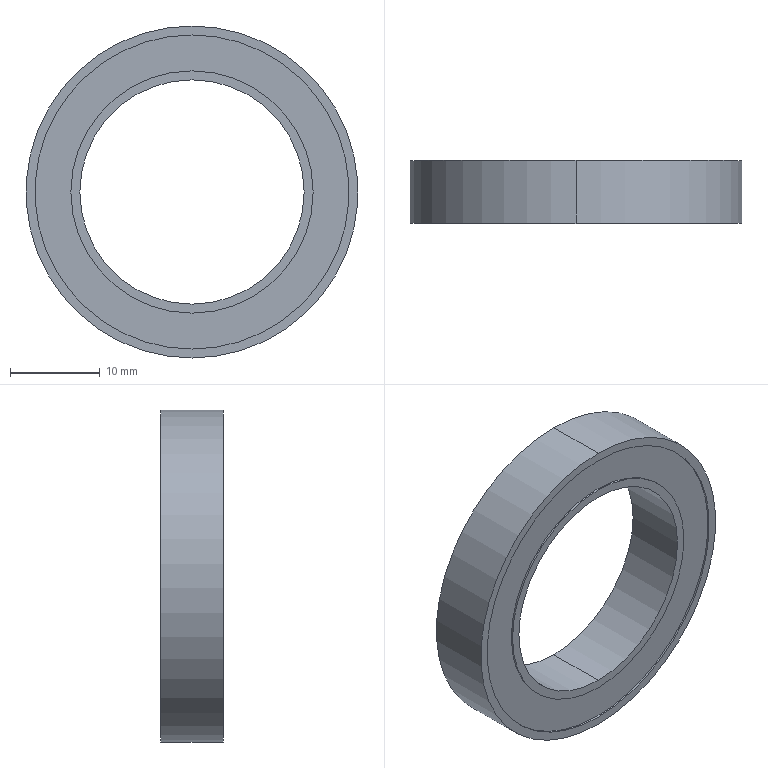Part | SolidWorks | features ICE 2, Extrusion 1 | 1 solid | 18 faces | box 37 x 7 x 37 mm | volume 3935 mm3 | cylinder 12 | plane 6 | commonest cylinder face diameters 27 x4 35 x4 25 x2 37 x2
STEP:
#1=CARTESIAN_POINT('',(0.,0.2,-13.5));
#2=VERTEX_POINT('',#1);
#3=CARTESIAN_POINT('',(0.,0.2,13.5));
#4=VERTEX_POINT('',#3);
#5=CARTESIAN_POINT('',(0.,0.2,0.));
#6=DIRECTION('',(0.,-1.,0.));
#7=DIRECTION('',(0.,0.,-1.));
#8=AXIS2_PLACEMENT_3D('',#5,#6,#7);
#9=CIRCLE('',#8,13.5);
#10=EDGE_CURVE('',#2,#4,#9,.T.);
#11=ORIENTED_EDGE('',*,*,#10,.T.);
#12=CARTESIAN_POINT('',(0.,0.,13.5));
#13=VERTEX_POINT('',#12);
#14=CARTESIAN_POINT('',(0.,0.2,13.5));
#15=DIRECTION('',(0.,-1.,0.));
#16=VECTOR('',#15,1000.);
#17=LINE('',#14,#16);
#18=EDGE_CURVE('',#4,#13,#17,.T.);
#19=ORIENTED_EDGE('',*,*,#18,.T.);
#20=CARTESIAN_POINT('',(0.,0.,-13.5));
#21=VERTEX_POINT('',#20);
#22=CARTESIAN_POINT('',(0.,0.,0.));
#23=DIRECTION('',(0.,-1.,0.));
#24=DIRECTION('',(0.,0.,-1.));
#25=AXIS2_PLACEMENT_3D('',#22,#23,#24);
#26=CIRCLE('',#25,13.5);
#27=EDGE_CURVE('',#21,#13,#26,.T.);
#28=ORIENTED_EDGE('',*,*,#27,.F.);
#29=CARTESIAN_POINT('',(0.,0.2,-13.5));
#30=DIRECTION('',(0.,-1.,0.));
#31=VECTOR('',#30,1000.);
#32=LINE('',#29,#31);
#33=EDGE_CURVE('',#2,#21,#32,.T.);
#34=ORIENTED_EDGE('',*,*,#33,.F.);
#35=EDGE_LOOP('',(#11,#19,#28,#34));
#36=FACE_OUTER_BOUND('',#35,.T.);
#37=CARTESIAN_POINT('',(0.,0.2,0.));
#38=DIRECTION('',(0.,-1.,0.));
#39=DIRECTION('',(0.,0.,-1.));
#40=AXIS2_PLACEMENT_3D('',#37,#38,#39);
#41=CYLINDRICAL_SURFACE('',#40,13.5);
#42=ADVANCED_FACE('',(#36),#41,.T.);
#43=CARTESIAN_POINT('',(0.,0.2,17.5));
#44=VERTEX_POINT('',#43);
#45=CARTESIAN_POINT('',(0.,0.2,-17.5));
#46=VERTEX_POINT('',#45);
#47=CARTESIAN_POINT('',(0.,0.2,0.));
#48=DIRECTION('',(0.,-1.,0.));
#49=DIRECTION('',(0.,0.,-1.));
#50=AXIS2_PLACEMENT_3D('',#47,#48,#49);
#51=CIRCLE('',#50,17.5);
#52=EDGE_CURVE('',#44,#46,#51,.T.);
#53=ORIENTED_EDGE('',*,*,#52,.F.);
#54=CARTESIAN_POINT('',(0.,0.,17.5));
#55=VERTEX_POINT('',#54);
#56=CARTESIAN_POINT('',(0.,0.2,17.5));
#57=DIRECTION('',(0.,-1.,0.));
#58=VECTOR('',#57,1000.);
#59=LINE('',#56,#58);
#60=EDGE_CURVE('',#44,#55,#59,.T.);
#61=ORIENTED_EDGE('',*,*,#60,.T.);
#62=CARTESIAN_POINT('',(0.,0.,-17.5));
#63=VERTEX_POINT('',#62);
#64=CARTESIAN_POINT('',(0.,0.,0.));
#65=DIRECTION('',(0.,-1.,0.));
#66=DIRECTION('',(0.,0.,-1.));
#67=AXIS2_PLACEMENT_3D('',#64,#65,#66);
#68=CIRCLE('',#67,17.5);
#69=EDGE_CURVE('',#55,#63,#68,.T.);
#70=ORIENTED_EDGE('',*,*,#69,.T.);
#71=CARTESIAN_POINT('',(0.,0.2,-17.5));
#72=DIRECTION('',(0.,-1.,0.));
#73=VECTOR('',#72,1000.);
#74=LINE('',#71,#73);
#75=EDGE_CURVE('',#46,#63,#74,.T.);
#76=ORIENTED_EDGE('',*,*,#75,.F.);
#77=EDGE_LOOP('',(#53,#61,#70,#76));
#78=FACE_OUTER_BOUND('',#77,.T.);
#79=CARTESIAN_POINT('',(0.,0.2,0.));
#80=DIRECTION('',(0.,-1.,0.));
#81=DIRECTION('',(0.,0.,-1.));
#82=AXIS2_PLACEMENT_3D('',#79,#80,#81);
#83=CYLINDRICAL_SURFACE('',#82,17.5);
#84=ADVANCED_FACE('',(#78),#83,.F.);
#85=CARTESIAN_POINT('',(0.,6.8,13.5));
#86=VERTEX_POINT('',#85);
#87=CARTESIAN_POINT('',(0.,6.8,-13.5));
#88=VERTEX_POINT('',#87);
#89=CARTESIAN_POINT('',(0.,6.8,0.));
#90=DIRECTION('',(0.,1.,0.));
#91=DIRECTION('',(0.,0.,1.));
#92=AXIS2_PLACEMENT_3D('',#89,#90,#91);
#93=CIRCLE('',#92,13.5);
#94=EDGE_CURVE('',#86,#88,#93,.T.);
#95=ORIENTED_EDGE('',*,*,#94,.T.);
#96=CARTESIAN_POINT('',(0.,7.,-13.5));
#97=VERTEX_POINT('',#96);
#98=CARTESIAN_POINT('',(0.,6.8,-13.5));
#99=DIRECTION('',(0.,1.,0.));
#100=VECTOR('',#99,1000.);
#101=LINE('',#98,#100);
#102=EDGE_CURVE('',#88,#97,#101,.T.);
#103=ORIENTED_EDGE('',*,*,#102,.T.);
#104=CARTESIAN_POINT('',(0.,7.,13.5));
#105=VERTEX_POINT('',#104);
#106=CARTESIAN_POINT('',(0.,7.,0.));
#107=DIRECTION('',(0.,1.,0.));
#108=DIRECTION('',(0.,0.,1.));
#109=AXIS2_PLACEMENT_3D('',#106,#107,#108);
#110=CIRCLE('',#109,13.5);
#111=EDGE_CURVE('',#105,#97,#110,.T.);
#112=ORIENTED_EDGE('',*,*,#111,.F.);
#113=CARTESIAN_POINT('',(0.,6.8,13.5));
#114=DIRECTION('',(0.,1.,0.));
#115=VECTOR('',#114,1000.);
#116=LINE('',#113,#115);
#117=EDGE_CURVE('',#86,#105,#116,.T.);
#118=ORIENTED_EDGE('',*,*,#117,.F.);
#119=EDGE_LOOP('',(#95,#103,#112,#118));
#120=FACE_OUTER_BOUND('',#119,.T.);
#121=CARTESIAN_POINT('',(0.,6.8,0.));
#122=DIRECTION('',(0.,1.,0.));
#123=DIRECTION('',(0.,0.,1.));
#124=AXIS2_PLACEMENT_3D('',#121,#122,#123);
#125=CYLINDRICAL_SURFACE('',#124,13.5);
#126=ADVANCED_FACE('',(#120),#125,.T.);
#127=CARTESIAN_POINT('',(0.,6.8,-17.5));
#128=VERTEX_POINT('',#127);
#129=CARTESIAN_POINT('',(0.,6.8,17.5));
#130=VERTEX_POINT('',#129);
#131=CARTESIAN_POINT('',(0.,6.8,0.));
#132=DIRECTION('',(0.,1.,0.));
#133=DIRECTION('',(0.,0.,1.));
#134=AXIS2_PLACEMENT_3D('',#131,#132,#133);
#135=CIRCLE('',#134,17.5);
#136=EDGE_CURVE('',#128,#130,#135,.T.);
#137=ORIENTED_EDGE('',*,*,#136,.F.);
#138=CARTESIAN_POINT('',(0.,7.,-17.5));
#139=VERTEX_POINT('',#138);
#140=CARTESIAN_POINT('',(0.,6.8,-17.5));
#141=DIRECTION('',(0.,1.,0.));
#142=VECTOR('',#141,1000.);
#143=LINE('',#140,#142);
#144=EDGE_CURVE('',#128,#139,#143,.T.);
#145=ORIENTED_EDGE('',*,*,#144,.T.);
#146=CARTESIAN_POINT('',(0.,7.,17.5));
#147=VERTEX_POINT('',#146);
#148=CARTESIAN_POINT('',(0.,7.,0.));
#149=DIRECTION('',(0.,1.,0.));
#150=DIRECTION('',(0.,0.,1.));
#151=AXIS2_PLACEMENT_3D('',#148,#149,#150);
#152=CIRCLE('',#151,17.5);
#153=EDGE_CURVE('',#139,#147,#152,.T.);
#154=ORIENTED_EDGE('',*,*,#153,.T.);
#155=CARTESIAN_POINT('',(0.,6.8,17.5));
#156=DIRECTION('',(0.,1.,0.));
#157=VECTOR('',#156,1000.);
#158=LINE('',#155,#157);
#159=EDGE_CURVE('',#130,#147,#158,.T.);
#160=ORIENTED_EDGE('',*,*,#159,.F.);
#161=EDGE_LOOP('',(#137,#145,#154,#160));
#162=FACE_OUTER_BOUND('',#161,.T.);
#163=CARTESIAN_POINT('',(0.,6.8,0.));
#164=DIRECTION('',(0.,1.,0.));
#165=DIRECTION('',(0.,0.,1.));
#166=AXIS2_PLACEMENT_3D('',#163,#164,#165);
#167=CYLINDRICAL_SURFACE('',#166,17.5);
#168=ADVANCED_FACE('',(#162),#167,.F.);
#169=CARTESIAN_POINT('',(0.,7.,-12.5));
#170=VERTEX_POINT('',#169);
#171=CARTESIAN_POINT('',(0.,7.,12.5));
#172=VERTEX_POINT('',#171);
#173=CARTESIAN_POINT('',(0.,7.,0.));
#174=DIRECTION('',(0.,1.,0.));
#175=DIRECTION('',(0.,0.,1.));
#176=AXIS2_PLACEMENT_3D('',#173,#174,#175);
#177=CIRCLE('',#176,12.5);
#178=EDGE_CURVE('',#170,#172,#177,.T.);
#179=ORIENTED_EDGE('',*,*,#178,.T.);
#180=CARTESIAN_POINT('',(0.,0.,12.5));
#181=VERTEX_POINT('',#180);
#182=CARTESIAN_POINT('',(0.,7.,12.5));
#183=DIRECTION('',(0.,-1.,0.));
#184=VECTOR('',#183,1000.);
#185=LINE('',#182,#184);
#186=EDGE_CURVE('',#172,#181,#185,.T.);
#187=ORIENTED_EDGE('',*,*,#186,.T.);
#188=CARTESIAN_POINT('',(0.,0.,-12.5));
#189=VERTEX_POINT('',#188);
#190=CARTESIAN_POINT('',(0.,0.,0.));
#191=DIRECTION('',(0.,1.,0.));
#192=DIRECTION('',(0.,0.,1.));
#193=AXIS2_PLACEMENT_3D('',#190,#191,#192);
#194=CIRCLE('',#193,12.5);
#195=EDGE_CURVE('',#189,#181,#194,.T.);
#196=ORIENTED_EDGE('',*,*,#195,.F.);
#197=CARTESIAN_POINT('',(0.,7.,-12.5));
#198=DIRECTION('',(0.,-1.,0.));
#199=VECTOR('',#198,1000.);
#200=LINE('',#197,#199);
#201=EDGE_CURVE('',#170,#189,#200,.T.);
#202=ORIENTED_EDGE('',*,*,#201,.F.);
#203=EDGE_LOOP('',(#179,#187,#196,#202));
#204=FACE_OUTER_BOUND('',#203,.T.);
#205=CARTESIAN_POINT('',(0.,7.,0.));
#206=DIRECTION('',(0.,-1.,0.));
#207=DIRECTION('',(0.,0.,-1.));
#208=AXIS2_PLACEMENT_3D('',#205,#206,#207);
#209=CYLINDRICAL_SURFACE('',#208,12.5);
#210=ADVANCED_FACE('',(#204),#209,.F.);
#211=CARTESIAN_POINT('',(0.,7.,18.5));
#212=VERTEX_POINT('',#211);
#213=CARTESIAN_POINT('',(0.,7.,-18.5));
#214=VERTEX_POINT('',#213);
#215=CARTESIAN_POINT('',(0.,7.,0.));
#216=DIRECTION('',(0.,1.,0.));
#217=DIRECTION('',(0.,0.,1.));
#218=AXIS2_PLACEMENT_3D('',#215,#216,#217);
#219=CIRCLE('',#218,18.5);
#220=EDGE_CURVE('',#212,#214,#219,.T.);
#221=ORIENTED_EDGE('',*,*,#220,.F.);
#222=CARTESIAN_POINT('',(0.,0.,18.5));
#223=VERTEX_POINT('',#222);
#224=CARTESIAN_POINT('',(0.,7.,18.5));
#225=DIRECTION('',(0.,-1.,0.));
#226=VECTOR('',#225,1000.);
#227=LINE('',#224,#226);
#228=EDGE_CURVE('',#212,#223,#227,.T.);
#229=ORIENTED_EDGE('',*,*,#228,.T.);
#230=CARTESIAN_POINT('',(0.,0.,-18.5));
#231=VERTEX_POINT('',#230);
#232=CARTESIAN_POINT('',(0.,0.,0.));
#233=DIRECTION('',(0.,1.,0.));
#234=DIRECTION('',(0.,0.,1.));
#235=AXIS2_PLACEMENT_3D('',#232,#233,#234);
#236=CIRCLE('',#235,18.5);
#237=EDGE_CURVE('',#223,#231,#236,.T.);
#238=ORIENTED_EDGE('',*,*,#237,.T.);
#239=CARTESIAN_POINT('',(0.,7.,-18.5));
#240=DIRECTION('',(0.,-1.,0.));
#241=VECTOR('',#240,1000.);
#242=LINE('',#239,#241);
#243=EDGE_CURVE('',#214,#231,#242,.T.);
#244=ORIENTED_EDGE('',*,*,#243,.F.);
#245=EDGE_LOOP('',(#221,#229,#238,#244));
#246=FACE_OUTER_BOUND('',#245,.T.);
#247=CARTESIAN_POINT('',(0.,7.,0.));
#248=DIRECTION('',(0.,-1.,0.));
#249=DIRECTION('',(0.,0.,-1.));
#250=AXIS2_PLACEMENT_3D('',#247,#248,#249);
#251=CYLINDRICAL_SURFACE('',#250,18.5);
#252=ADVANCED_FACE('',(#246),#251,.T.);
#253=ORIENTED_EDGE('',*,*,#195,.T.);
#254=CARTESIAN_POINT('',(0.,0.,0.));
#255=DIRECTION('',(0.,1.,0.));
#256=DIRECTION('',(0.,0.,1.));
#257=AXIS2_PLACEMENT_3D('',#254,#255,#256);
#258=CIRCLE('',#257,12.5);
#259=EDGE_CURVE('',#181,#189,#258,.T.);
#260=ORIENTED_EDGE('',*,*,#259,.T.);
#261=EDGE_LOOP('',(#253,#260));
#262=FACE_BOUND('',#261,.T.);
#263=ORIENTED_EDGE('',*,*,#27,.T.);
#264=CARTESIAN_POINT('',(0.,0.,0.));
#265=DIRECTION('',(0.,-1.,0.));
#266=DIRECTION('',(0.,0.,-1.));
#267=AXIS2_PLACEMENT_3D('',#264,#265,#266);
#268=CIRCLE('',#267,13.5);
#269=EDGE_CURVE('',#13,#21,#268,.T.);
#270=ORIENTED_EDGE('',*,*,#269,.T.);
#271=EDGE_LOOP('',(#263,#270));
#272=FACE_OUTER_BOUND('',#271,.T.);
#273=CARTESIAN_POINT('',(0.,0.,0.));
#274=DIRECTION('',(0.,1.,0.));
#275=DIRECTION('',(0.,0.,1.));
#276=AXIS2_PLACEMENT_3D('',#273,#274,#275);
#277=PLANE('',#276);
#278=ADVANCED_FACE('',(#262,#272),#277,.F.);
#279=ORIENTED_EDGE('',*,*,#178,.F.);
#280=CARTESIAN_POINT('',(0.,7.,0.));
#281=DIRECTION('',(0.,1.,0.));
#282=DIRECTION('',(0.,0.,1.));
#283=AXIS2_PLACEMENT_3D('',#280,#281,#282);
#284=CIRCLE('',#283,12.5);
#285=EDGE_CURVE('',#172,#170,#284,.T.);
#286=ORIENTED_EDGE('',*,*,#285,.F.);
#287=EDGE_LOOP('',(#279,#286));
#288=FACE_BOUND('',#287,.T.);
#289=ORIENTED_EDGE('',*,*,#111,.T.);
#290=CARTESIAN_POINT('',(0.,7.,0.));
#291=DIRECTION('',(0.,1.,0.));
#292=DIRECTION('',(0.,0.,1.));
#293=AXIS2_PLACEMENT_3D('',#290,#291,#292);
#294=CIRCLE('',#293,13.5);
#295=EDGE_CURVE('',#97,#105,#294,.T.);
#296=ORIENTED_EDGE('',*,*,#295,.T.);
#297=EDGE_LOOP('',(#289,#296));
#298=FACE_OUTER_BOUND('',#297,.T.);
#299=CARTESIAN_POINT('',(0.,7.,0.));
#300=DIRECTION('',(0.,1.,0.));
#301=DIRECTION('',(0.,0.,1.));
#302=AXIS2_PLACEMENT_3D('',#299,#300,#301);
#303=PLANE('',#302);
#304=ADVANCED_FACE('',(#288,#298),#303,.T.);
#305=CARTESIAN_POINT('',(0.,7.,0.));
#306=DIRECTION('',(0.,1.,0.));
#307=DIRECTION('',(0.,0.,1.));
#308=AXIS2_PLACEMENT_3D('',#305,#306,#307);
#309=CIRCLE('',#308,17.5);
#310=EDGE_CURVE('',#147,#139,#309,.T.);
#311=ORIENTED_EDGE('',*,*,#310,.F.);
#312=ORIENTED_EDGE('',*,*,#153,.F.);
#313=EDGE_LOOP('',(#311,#312));
#314=FACE_BOUND('',#313,.T.);
#315=CARTESIAN_POINT('',(0.,7.,0.));
#316=DIRECTION('',(0.,1.,0.));
#317=DIRECTION('',(0.,0.,1.));
#318=AXIS2_PLACEMENT_3D('',#315,#316,#317);
#319=CIRCLE('',#318,18.5);
#320=EDGE_CURVE('',#214,#212,#319,.T.);
#321=ORIENTED_EDGE('',*,*,#320,.T.);
#322=ORIENTED_EDGE('',*,*,#220,.T.);
#323=EDGE_LOOP('',(#321,#322));
#324=FACE_OUTER_BOUND('',#323,.T.);
#325=CARTESIAN_POINT('',(0.,7.,0.));
#326=DIRECTION('',(0.,1.,0.));
#327=DIRECTION('',(0.,0.,1.));
#328=AXIS2_PLACEMENT_3D('',#325,#326,#327);
#329=PLANE('',#328);
#330=ADVANCED_FACE('',(#314,#324),#329,.T.);
#331=CARTESIAN_POINT('',(0.,0.,0.));
#332=DIRECTION('',(0.,-1.,0.));
#333=DIRECTION('',(0.,0.,-1.));
#334=AXIS2_PLACEMENT_3D('',#331,#332,#333);
#335=CIRCLE('',#334,17.5);
#336=EDGE_CURVE('',#63,#55,#335,.T.);
#337=ORIENTED_EDGE('',*,*,#336,.F.);
#338=ORIENTED_EDGE('',*,*,#69,.F.);
#339=EDGE_LOOP('',(#337,#338));
#340=FACE_BOUND('',#339,.T.);
#341=CARTESIAN_POINT('',(0.,0.,0.));
#342=DIRECTION('',(0.,1.,0.));
#343=DIRECTION('',(0.,0.,1.));
#344=AXIS2_PLACEMENT_3D('',#341,#342,#343);
#345=CIRCLE('',#344,18.5);
#346=EDGE_CURVE('',#231,#223,#345,.T.);
#347=ORIENTED_EDGE('',*,*,#346,.F.);
#348=ORIENTED_EDGE('',*,*,#237,.F.);
#349=EDGE_LOOP('',(#347,#348));
#350=FACE_OUTER_BOUND('',#349,.T.);
#351=CARTESIAN_POINT('',(0.,0.,0.));
#352=DIRECTION('',(0.,1.,0.));
#353=DIRECTION('',(0.,0.,1.));
#354=AXIS2_PLACEMENT_3D('',#351,#352,#353);
#355=PLANE('',#354);
#356=ADVANCED_FACE('',(#340,#350),#355,.F.);
#357=ORIENTED_EDGE('',*,*,#228,.F.);
#358=ORIENTED_EDGE('',*,*,#320,.F.);
#359=ORIENTED_EDGE('',*,*,#243,.T.);
#360=ORIENTED_EDGE('',*,*,#346,.T.);
#361=EDGE_LOOP('',(#357,#358,#359,#360));
#362=FACE_OUTER_BOUND('',#361,.T.);
#363=CARTESIAN_POINT('',(0.,7.,0.));
#364=DIRECTION('',(0.,-1.,0.));
#365=DIRECTION('',(0.,0.,-1.));
#366=AXIS2_PLACEMENT_3D('',#363,#364,#365);
#367=CYLINDRICAL_SURFACE('',#366,18.5);
#368=ADVANCED_FACE('',(#362),#367,.T.);
#369=ORIENTED_EDGE('',*,*,#186,.F.);
#370=ORIENTED_EDGE('',*,*,#285,.T.);
#371=ORIENTED_EDGE('',*,*,#201,.T.);
#372=ORIENTED_EDGE('',*,*,#259,.F.);
#373=EDGE_LOOP('',(#369,#370,#371,#372));
#374=FACE_OUTER_BOUND('',#373,.T.);
#375=CARTESIAN_POINT('',(0.,7.,0.));
#376=DIRECTION('',(0.,-1.,0.));
#377=DIRECTION('',(0.,0.,-1.));
#378=AXIS2_PLACEMENT_3D('',#375,#376,#377);
#379=CYLINDRICAL_SURFACE('',#378,12.5);
#380=ADVANCED_FACE('',(#374),#379,.F.);
#381=ORIENTED_EDGE('',*,*,#144,.F.);
#382=CARTESIAN_POINT('',(0.,6.8,0.));
#383=DIRECTION('',(0.,1.,0.));
#384=DIRECTION('',(0.,0.,1.));
#385=AXIS2_PLACEMENT_3D('',#382,#383,#384);
#386=CIRCLE('',#385,17.5);
#387=EDGE_CURVE('',#130,#128,#386,.T.);
#388=ORIENTED_EDGE('',*,*,#387,.F.);
#389=ORIENTED_EDGE('',*,*,#159,.T.);
#390=ORIENTED_EDGE('',*,*,#310,.T.);
#391=EDGE_LOOP('',(#381,#388,#389,#390));
#392=FACE_OUTER_BOUND('',#391,.T.);
#393=CARTESIAN_POINT('',(0.,6.8,0.));
#394=DIRECTION('',(0.,1.,0.));
#395=DIRECTION('',(0.,0.,1.));
#396=AXIS2_PLACEMENT_3D('',#393,#394,#395);
#397=CYLINDRICAL_SURFACE('',#396,17.5);
#398=ADVANCED_FACE('',(#392),#397,.F.);
#399=ORIENTED_EDGE('',*,*,#94,.F.);
#400=CARTESIAN_POINT('',(0.,6.8,0.));
#401=DIRECTION('',(0.,1.,0.));
#402=DIRECTION('',(0.,0.,1.));
#403=AXIS2_PLACEMENT_3D('',#400,#401,#402);
#404=CIRCLE('',#403,13.5);
#405=EDGE_CURVE('',#88,#86,#404,.T.);
#406=ORIENTED_EDGE('',*,*,#405,.F.);
#407=EDGE_LOOP('',(#399,#406));
#408=FACE_BOUND('',#407,.T.);
#409=ORIENTED_EDGE('',*,*,#387,.T.);
#410=ORIENTED_EDGE('',*,*,#136,.T.);
#411=EDGE_LOOP('',(#409,#410));
#412=FACE_OUTER_BOUND('',#411,.T.);
#413=CARTESIAN_POINT('',(0.,6.8,0.));
#414=DIRECTION('',(0.,1.,0.));
#415=DIRECTION('',(0.,0.,1.));
#416=AXIS2_PLACEMENT_3D('',#413,#414,#415);
#417=PLANE('',#416);
#418=ADVANCED_FACE('',(#408,#412),#417,.T.);
#419=ORIENTED_EDGE('',*,*,#102,.F.);
#420=ORIENTED_EDGE('',*,*,#405,.T.);
#421=ORIENTED_EDGE('',*,*,#117,.T.);
#422=ORIENTED_EDGE('',*,*,#295,.F.);
#423=EDGE_LOOP('',(#419,#420,#421,#422));
#424=FACE_OUTER_BOUND('',#423,.T.);
#425=CARTESIAN_POINT('',(0.,6.8,0.));
#426=DIRECTION('',(0.,1.,0.));
#427=DIRECTION('',(0.,0.,1.));
#428=AXIS2_PLACEMENT_3D('',#425,#426,#427);
#429=CYLINDRICAL_SURFACE('',#428,13.5);
#430=ADVANCED_FACE('',(#424),#429,.T.);
#431=ORIENTED_EDGE('',*,*,#60,.F.);
#432=CARTESIAN_POINT('',(0.,0.2,0.));
#433=DIRECTION('',(0.,-1.,0.));
#434=DIRECTION('',(0.,0.,-1.));
#435=AXIS2_PLACEMENT_3D('',#432,#433,#434);
#436=CIRCLE('',#435,17.5);
#437=EDGE_CURVE('',#46,#44,#436,.T.);
#438=ORIENTED_EDGE('',*,*,#437,.F.);
#439=ORIENTED_EDGE('',*,*,#75,.T.);
#440=ORIENTED_EDGE('',*,*,#336,.T.);
#441=EDGE_LOOP('',(#431,#438,#439,#440));
#442=FACE_OUTER_BOUND('',#441,.T.);
#443=CARTESIAN_POINT('',(0.,0.2,0.));
#444=DIRECTION('',(0.,-1.,0.));
#445=DIRECTION('',(0.,0.,-1.));
#446=AXIS2_PLACEMENT_3D('',#443,#444,#445);
#447=CYLINDRICAL_SURFACE('',#446,17.5);
#448=ADVANCED_FACE('',(#442),#447,.F.);
#449=ORIENTED_EDGE('',*,*,#10,.F.);
#450=CARTESIAN_POINT('',(0.,0.2,0.));
#451=DIRECTION('',(0.,-1.,0.));
#452=DIRECTION('',(0.,0.,-1.));
#453=AXIS2_PLACEMENT_3D('',#450,#451,#452);
#454=CIRCLE('',#453,13.5);
#455=EDGE_CURVE('',#4,#2,#454,.T.);
#456=ORIENTED_EDGE('',*,*,#455,.F.);
#457=EDGE_LOOP('',(#449,#456));
#458=FACE_BOUND('',#457,.T.);
#459=ORIENTED_EDGE('',*,*,#437,.T.);
#460=ORIENTED_EDGE('',*,*,#52,.T.);
#461=EDGE_LOOP('',(#459,#460));
#462=FACE_OUTER_BOUND('',#461,.T.);
#463=CARTESIAN_POINT('',(0.,0.2,0.));
#464=DIRECTION('',(0.,-1.,0.));
#465=DIRECTION('',(0.,0.,-1.));
#466=AXIS2_PLACEMENT_3D('',#463,#464,#465);
#467=PLANE('',#466);
#468=ADVANCED_FACE('',(#458,#462),#467,.T.);
#469=ORIENTED_EDGE('',*,*,#18,.F.);
#470=ORIENTED_EDGE('',*,*,#455,.T.);
#471=ORIENTED_EDGE('',*,*,#33,.T.);
#472=ORIENTED_EDGE('',*,*,#269,.F.);
#473=EDGE_LOOP('',(#469,#470,#471,#472));
#474=FACE_OUTER_BOUND('',#473,.T.);
#475=CARTESIAN_POINT('',(0.,0.2,0.));
#476=DIRECTION('',(0.,-1.,0.));
#477=DIRECTION('',(0.,0.,-1.));
#478=AXIS2_PLACEMENT_3D('',#475,#476,#477);
#479=CYLINDRICAL_SURFACE('',#478,13.5);
#480=ADVANCED_FACE('',(#474),#479,.T.);
#481=CLOSED_SHELL('',(#42,#84,#126,#168,#210,#252,#278,#304,#330,#356,#368,#380,#398,#418,#430,#448,#468,#480));
#482=MANIFOLD_SOLID_BREP('',#481);
#483=CARTESIAN_POINT('',(0.,0.,0.));
#484=DIRECTION('',(0.,0.,1.));
#485=DIRECTION('',(1.,0.,0.));
#486=AXIS2_PLACEMENT_3D('',#483,#484,#485);
#487=(LENGTH_UNIT()NAMED_UNIT(*)SI_UNIT(.MILLI.,.METRE.));
#488=UNCERTAINTY_MEASURE_WITH_UNIT(LENGTH_MEASURE(0.00001),#487,'','');
#489=(NAMED_UNIT(*)PLANE_ANGLE_UNIT()SI_UNIT($,.RADIAN.));
#490=(NAMED_UNIT(*)SI_UNIT($,.STERADIAN.)SOLID_ANGLE_UNIT());
#491=(GEOMETRIC_REPRESENTATION_CONTEXT(3)GLOBAL_UNCERTAINTY_ASSIGNED_CONTEXT((#488))GLOBAL_UNIT_ASSIGNED_CONTEXT((#487,#489,#490))REPRESENTATION_CONTEXT('',''));
#492=ADVANCED_BREP_SHAPE_REPRESENTATION('',(#482,#486),#491);